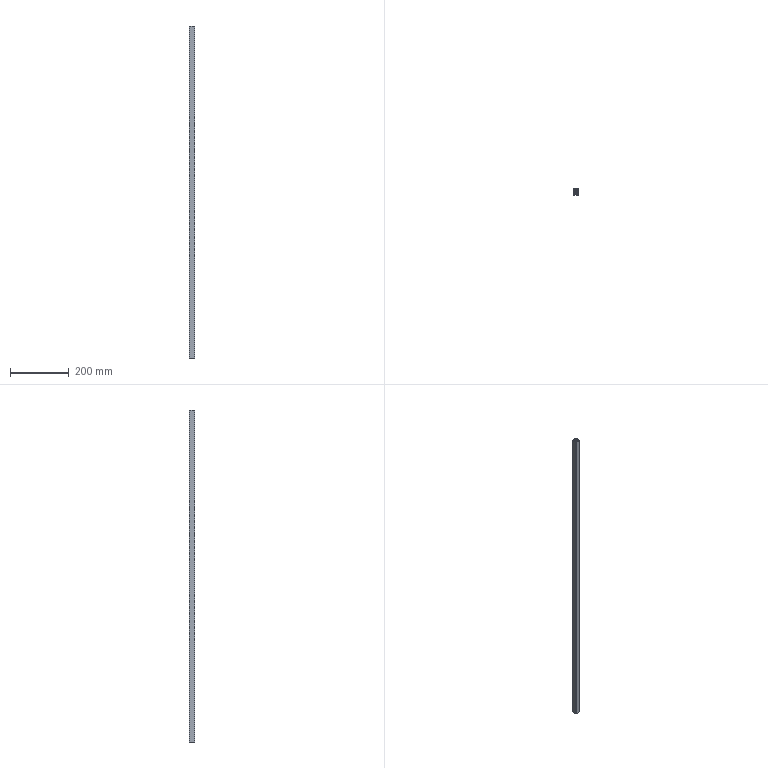Part | SolidWorks | features Extrusion 1 | 1 solid | 72 faces | box 20 x 20 x 1135 mm | volume 223287 mm3 | plane 38 | cylinder 34 | commonest cylinder face diameters 0.6 x20 4 x8 3 x4 5 x2